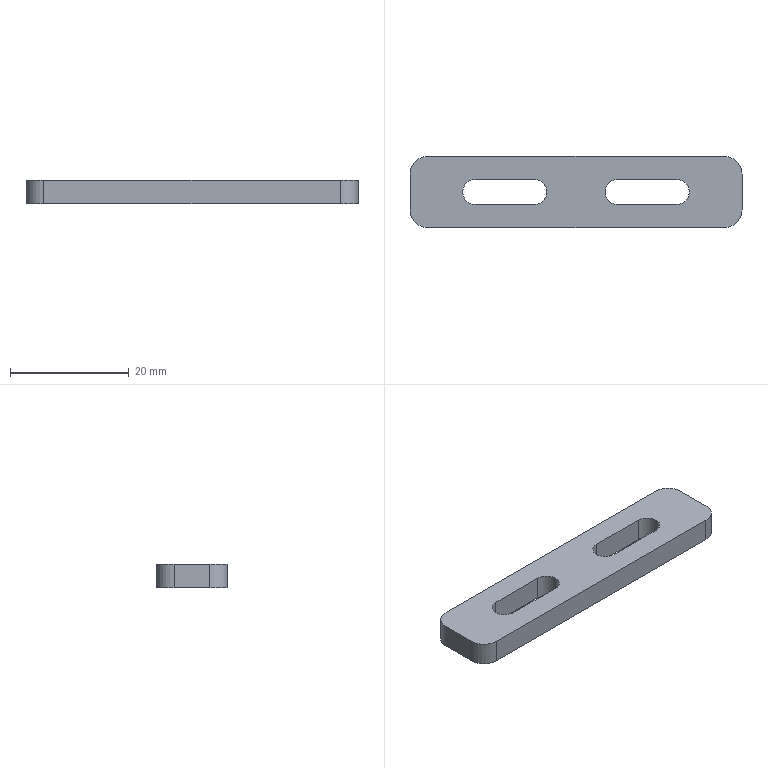Part | STEP file | 001-011-Blanking flip sensor mounting seat | 1 solid | 20 faces | box 56 x 12 x 4 mm | volume 2210 mm3 | cylinder 10 | plane 10 | commonest cylinder face diameters 4.2 x6 6 x4